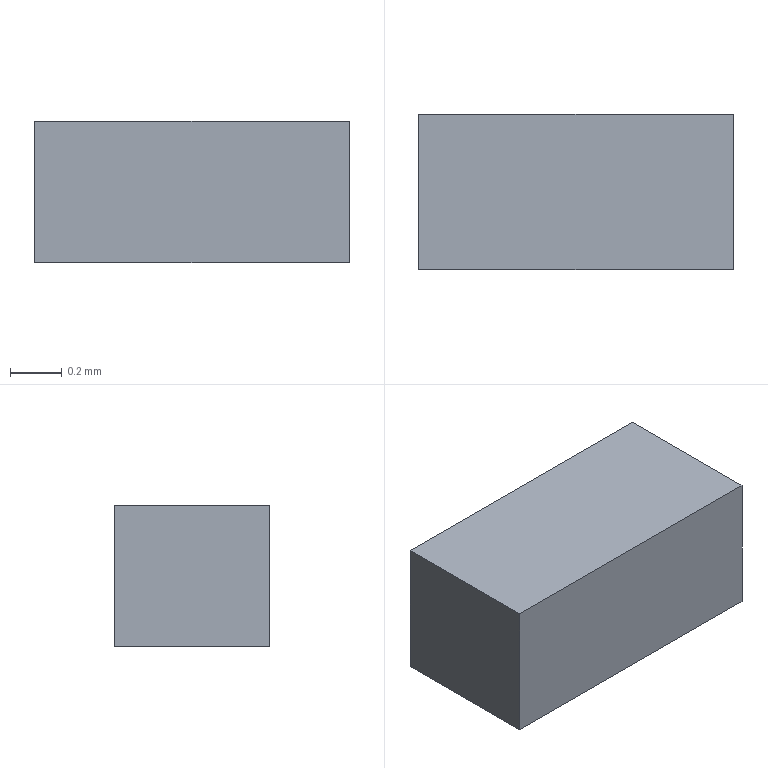Part | Creo | 1 solid | 6 faces | box 1.218 x 0.6006 x 0.55 mm | volume 0.4024 mm3 | plane 6
STEP:
#1=CARTESIAN_POINT('',(0.,0.,0.));
#2=DIRECTION('',(0.,0.,1.));
#3=DIRECTION('',(1.,0.,0.));
#4=AXIS2_PLACEMENT_3D('',#1,#2,#3);
#5=CARTESIAN_POINT('',(-0.6098,0.2998,0.));
#6=VERTEX_POINT('',#5);
#7=CARTESIAN_POINT('',(-0.6098,-0.3009,0.));
#8=VERTEX_POINT('',#7);
#9=CARTESIAN_POINT('',(-0.6098,0.2998,0.));
#10=DIRECTION('',(0.,-1.,0.));
#11=VECTOR('',#10,0.6006);
#12=LINE('',#9,#11);
#13=EDGE_CURVE('',#6,#8,#12,.T.);
#14=ORIENTED_EDGE('',*,*,#13,.T.);
#15=CARTESIAN_POINT('',(0.6081,-0.3009,0.));
#16=VERTEX_POINT('',#15);
#17=CARTESIAN_POINT('',(-0.6098,-0.3009,0.));
#18=DIRECTION('',(1.,0.,0.));
#19=VECTOR('',#18,1.218);
#20=LINE('',#17,#19);
#21=EDGE_CURVE('',#8,#16,#20,.T.);
#22=ORIENTED_EDGE('',*,*,#21,.T.);
#23=CARTESIAN_POINT('',(0.6081,0.2998,0.));
#24=VERTEX_POINT('',#23);
#25=CARTESIAN_POINT('',(0.6081,-0.3009,0.));
#26=DIRECTION('',(0.,1.,0.));
#27=VECTOR('',#26,0.6006);
#28=LINE('',#25,#27);
#29=EDGE_CURVE('',#16,#24,#28,.T.);
#30=ORIENTED_EDGE('',*,*,#29,.T.);
#31=CARTESIAN_POINT('',(0.6081,0.2998,0.));
#32=DIRECTION('',(-1.,0.,0.));
#33=VECTOR('',#32,1.218);
#34=LINE('',#31,#33);
#35=EDGE_CURVE('',#24,#6,#34,.T.);
#36=ORIENTED_EDGE('',*,*,#35,.T.);
#37=EDGE_LOOP('',(#14,#22,#30,#36));
#38=FACE_OUTER_BOUND('',#37,.F.);
#39=CARTESIAN_POINT('',(0.,0.,0.));
#40=DIRECTION('',(0.,0.,1.));
#41=DIRECTION('',(1.,0.,0.));
#42=AXIS2_PLACEMENT_3D('',#39,#40,#41);
#43=PLANE('',#42);
#44=ADVANCED_FACE('',(#38),#43,.F.);
#45=ORIENTED_EDGE('',*,*,#13,.F.);
#46=CARTESIAN_POINT('',(-0.6098,0.2998,0.55));
#47=VERTEX_POINT('',#46);
#48=CARTESIAN_POINT('',(-0.6098,0.2998,0.));
#49=DIRECTION('',(0.,0.,1.));
#50=VECTOR('',#49,0.55);
#51=LINE('',#48,#50);
#52=EDGE_CURVE('',#6,#47,#51,.T.);
#53=ORIENTED_EDGE('',*,*,#52,.T.);
#54=CARTESIAN_POINT('',(-0.6098,-0.3009,0.55));
#55=VERTEX_POINT('',#54);
#56=CARTESIAN_POINT('',(-0.6098,0.2998,0.55));
#57=DIRECTION('',(0.,-1.,0.));
#58=VECTOR('',#57,0.6006);
#59=LINE('',#56,#58);
#60=EDGE_CURVE('',#47,#55,#59,.T.);
#61=ORIENTED_EDGE('',*,*,#60,.T.);
#62=CARTESIAN_POINT('',(-0.6098,-0.3009,0.));
#63=DIRECTION('',(0.,0.,1.));
#64=VECTOR('',#63,0.55);
#65=LINE('',#62,#64);
#66=EDGE_CURVE('',#8,#55,#65,.T.);
#67=ORIENTED_EDGE('',*,*,#66,.F.);
#68=EDGE_LOOP('',(#45,#53,#61,#67));
#69=FACE_OUTER_BOUND('',#68,.F.);
#70=CARTESIAN_POINT('',(-0.6098,0.2998,0.));
#71=DIRECTION('',(-1.,0.,0.));
#72=DIRECTION('',(0.,-1.,0.));
#73=AXIS2_PLACEMENT_3D('',#70,#71,#72);
#74=PLANE('',#73);
#75=ADVANCED_FACE('',(#69),#74,.T.);
#76=ORIENTED_EDGE('',*,*,#35,.F.);
#77=CARTESIAN_POINT('',(0.6081,0.2998,0.55));
#78=VERTEX_POINT('',#77);
#79=CARTESIAN_POINT('',(0.6081,0.2998,0.));
#80=DIRECTION('',(0.,0.,1.));
#81=VECTOR('',#80,0.55);
#82=LINE('',#79,#81);
#83=EDGE_CURVE('',#24,#78,#82,.T.);
#84=ORIENTED_EDGE('',*,*,#83,.T.);
#85=CARTESIAN_POINT('',(0.6081,0.2998,0.55));
#86=DIRECTION('',(-1.,0.,0.));
#87=VECTOR('',#86,1.218);
#88=LINE('',#85,#87);
#89=EDGE_CURVE('',#78,#47,#88,.T.);
#90=ORIENTED_EDGE('',*,*,#89,.T.);
#91=ORIENTED_EDGE('',*,*,#52,.F.);
#92=EDGE_LOOP('',(#76,#84,#90,#91));
#93=FACE_OUTER_BOUND('',#92,.F.);
#94=CARTESIAN_POINT('',(0.6081,0.2998,0.));
#95=DIRECTION('',(0.,1.,0.));
#96=DIRECTION('',(-1.,0.,0.));
#97=AXIS2_PLACEMENT_3D('',#94,#95,#96);
#98=PLANE('',#97);
#99=ADVANCED_FACE('',(#93),#98,.T.);
#100=ORIENTED_EDGE('',*,*,#29,.F.);
#101=CARTESIAN_POINT('',(0.6081,-0.3009,0.55));
#102=VERTEX_POINT('',#101);
#103=CARTESIAN_POINT('',(0.6081,-0.3009,0.));
#104=DIRECTION('',(0.,0.,1.));
#105=VECTOR('',#104,0.55);
#106=LINE('',#103,#105);
#107=EDGE_CURVE('',#16,#102,#106,.T.);
#108=ORIENTED_EDGE('',*,*,#107,.T.);
#109=CARTESIAN_POINT('',(0.6081,-0.3009,0.55));
#110=DIRECTION('',(0.,1.,0.));
#111=VECTOR('',#110,0.6006);
#112=LINE('',#109,#111);
#113=EDGE_CURVE('',#102,#78,#112,.T.);
#114=ORIENTED_EDGE('',*,*,#113,.T.);
#115=ORIENTED_EDGE('',*,*,#83,.F.);
#116=EDGE_LOOP('',(#100,#108,#114,#115));
#117=FACE_OUTER_BOUND('',#116,.F.);
#118=CARTESIAN_POINT('',(0.6081,-0.3009,0.));
#119=DIRECTION('',(1.,0.,0.));
#120=DIRECTION('',(0.,1.,0.));
#121=AXIS2_PLACEMENT_3D('',#118,#119,#120);
#122=PLANE('',#121);
#123=ADVANCED_FACE('',(#117),#122,.T.);
#124=ORIENTED_EDGE('',*,*,#21,.F.);
#125=ORIENTED_EDGE('',*,*,#66,.T.);
#126=CARTESIAN_POINT('',(-0.6098,-0.3009,0.55));
#127=DIRECTION('',(1.,0.,0.));
#128=VECTOR('',#127,1.218);
#129=LINE('',#126,#128);
#130=EDGE_CURVE('',#55,#102,#129,.T.);
#131=ORIENTED_EDGE('',*,*,#130,.T.);
#132=ORIENTED_EDGE('',*,*,#107,.F.);
#133=EDGE_LOOP('',(#124,#125,#131,#132));
#134=FACE_OUTER_BOUND('',#133,.F.);
#135=CARTESIAN_POINT('',(-0.6098,-0.3009,0.));
#136=DIRECTION('',(0.,-1.,0.));
#137=DIRECTION('',(1.,0.,0.));
#138=AXIS2_PLACEMENT_3D('',#135,#136,#137);
#139=PLANE('',#138);
#140=ADVANCED_FACE('',(#134),#139,.T.);
#141=ORIENTED_EDGE('',*,*,#60,.F.);
#142=ORIENTED_EDGE('',*,*,#89,.F.);
#143=ORIENTED_EDGE('',*,*,#113,.F.);
#144=ORIENTED_EDGE('',*,*,#130,.F.);
#145=EDGE_LOOP('',(#141,#142,#143,#144));
#146=FACE_OUTER_BOUND('',#145,.F.);
#147=CARTESIAN_POINT('',(0.,0.,0.55));
#148=DIRECTION('',(0.,0.,1.));
#149=DIRECTION('',(1.,0.,0.));
#150=AXIS2_PLACEMENT_3D('',#147,#148,#149);
#151=PLANE('',#150);
#152=ADVANCED_FACE('',(#146),#151,.T.);
#153=CLOSED_SHELL('',(#44,#75,#99,#123,#140,#152));
#154=MANIFOLD_SOLID_BREP('',#153);
#155=(LENGTH_UNIT()NAMED_UNIT(*)SI_UNIT(.MILLI.,.METRE.));
#156=UNCERTAINTY_MEASURE_WITH_UNIT(LENGTH_MEASURE(0.0001465),#155,'','');
#157=(NAMED_UNIT(*)PLANE_ANGLE_UNIT()SI_UNIT($,.RADIAN.));
#158=PLANE_ANGLE_MEASURE_WITH_UNIT(PLANE_ANGLE_MEASURE(0.01745),#157);
#159=(CONVERSION_BASED_UNIT('DEGREE',#158)NAMED_UNIT(*)PLANE_ANGLE_UNIT());
#160=(NAMED_UNIT(*)SI_UNIT($,.STERADIAN.)SOLID_ANGLE_UNIT());
#161=(GEOMETRIC_REPRESENTATION_CONTEXT(3)GLOBAL_UNCERTAINTY_ASSIGNED_CONTEXT((#156))GLOBAL_UNIT_ASSIGNED_CONTEXT((#155,#159,#160))REPRESENTATION_CONTEXT('',''));
#162=ADVANCED_BREP_SHAPE_REPRESENTATION('',(#4,#154),#161);